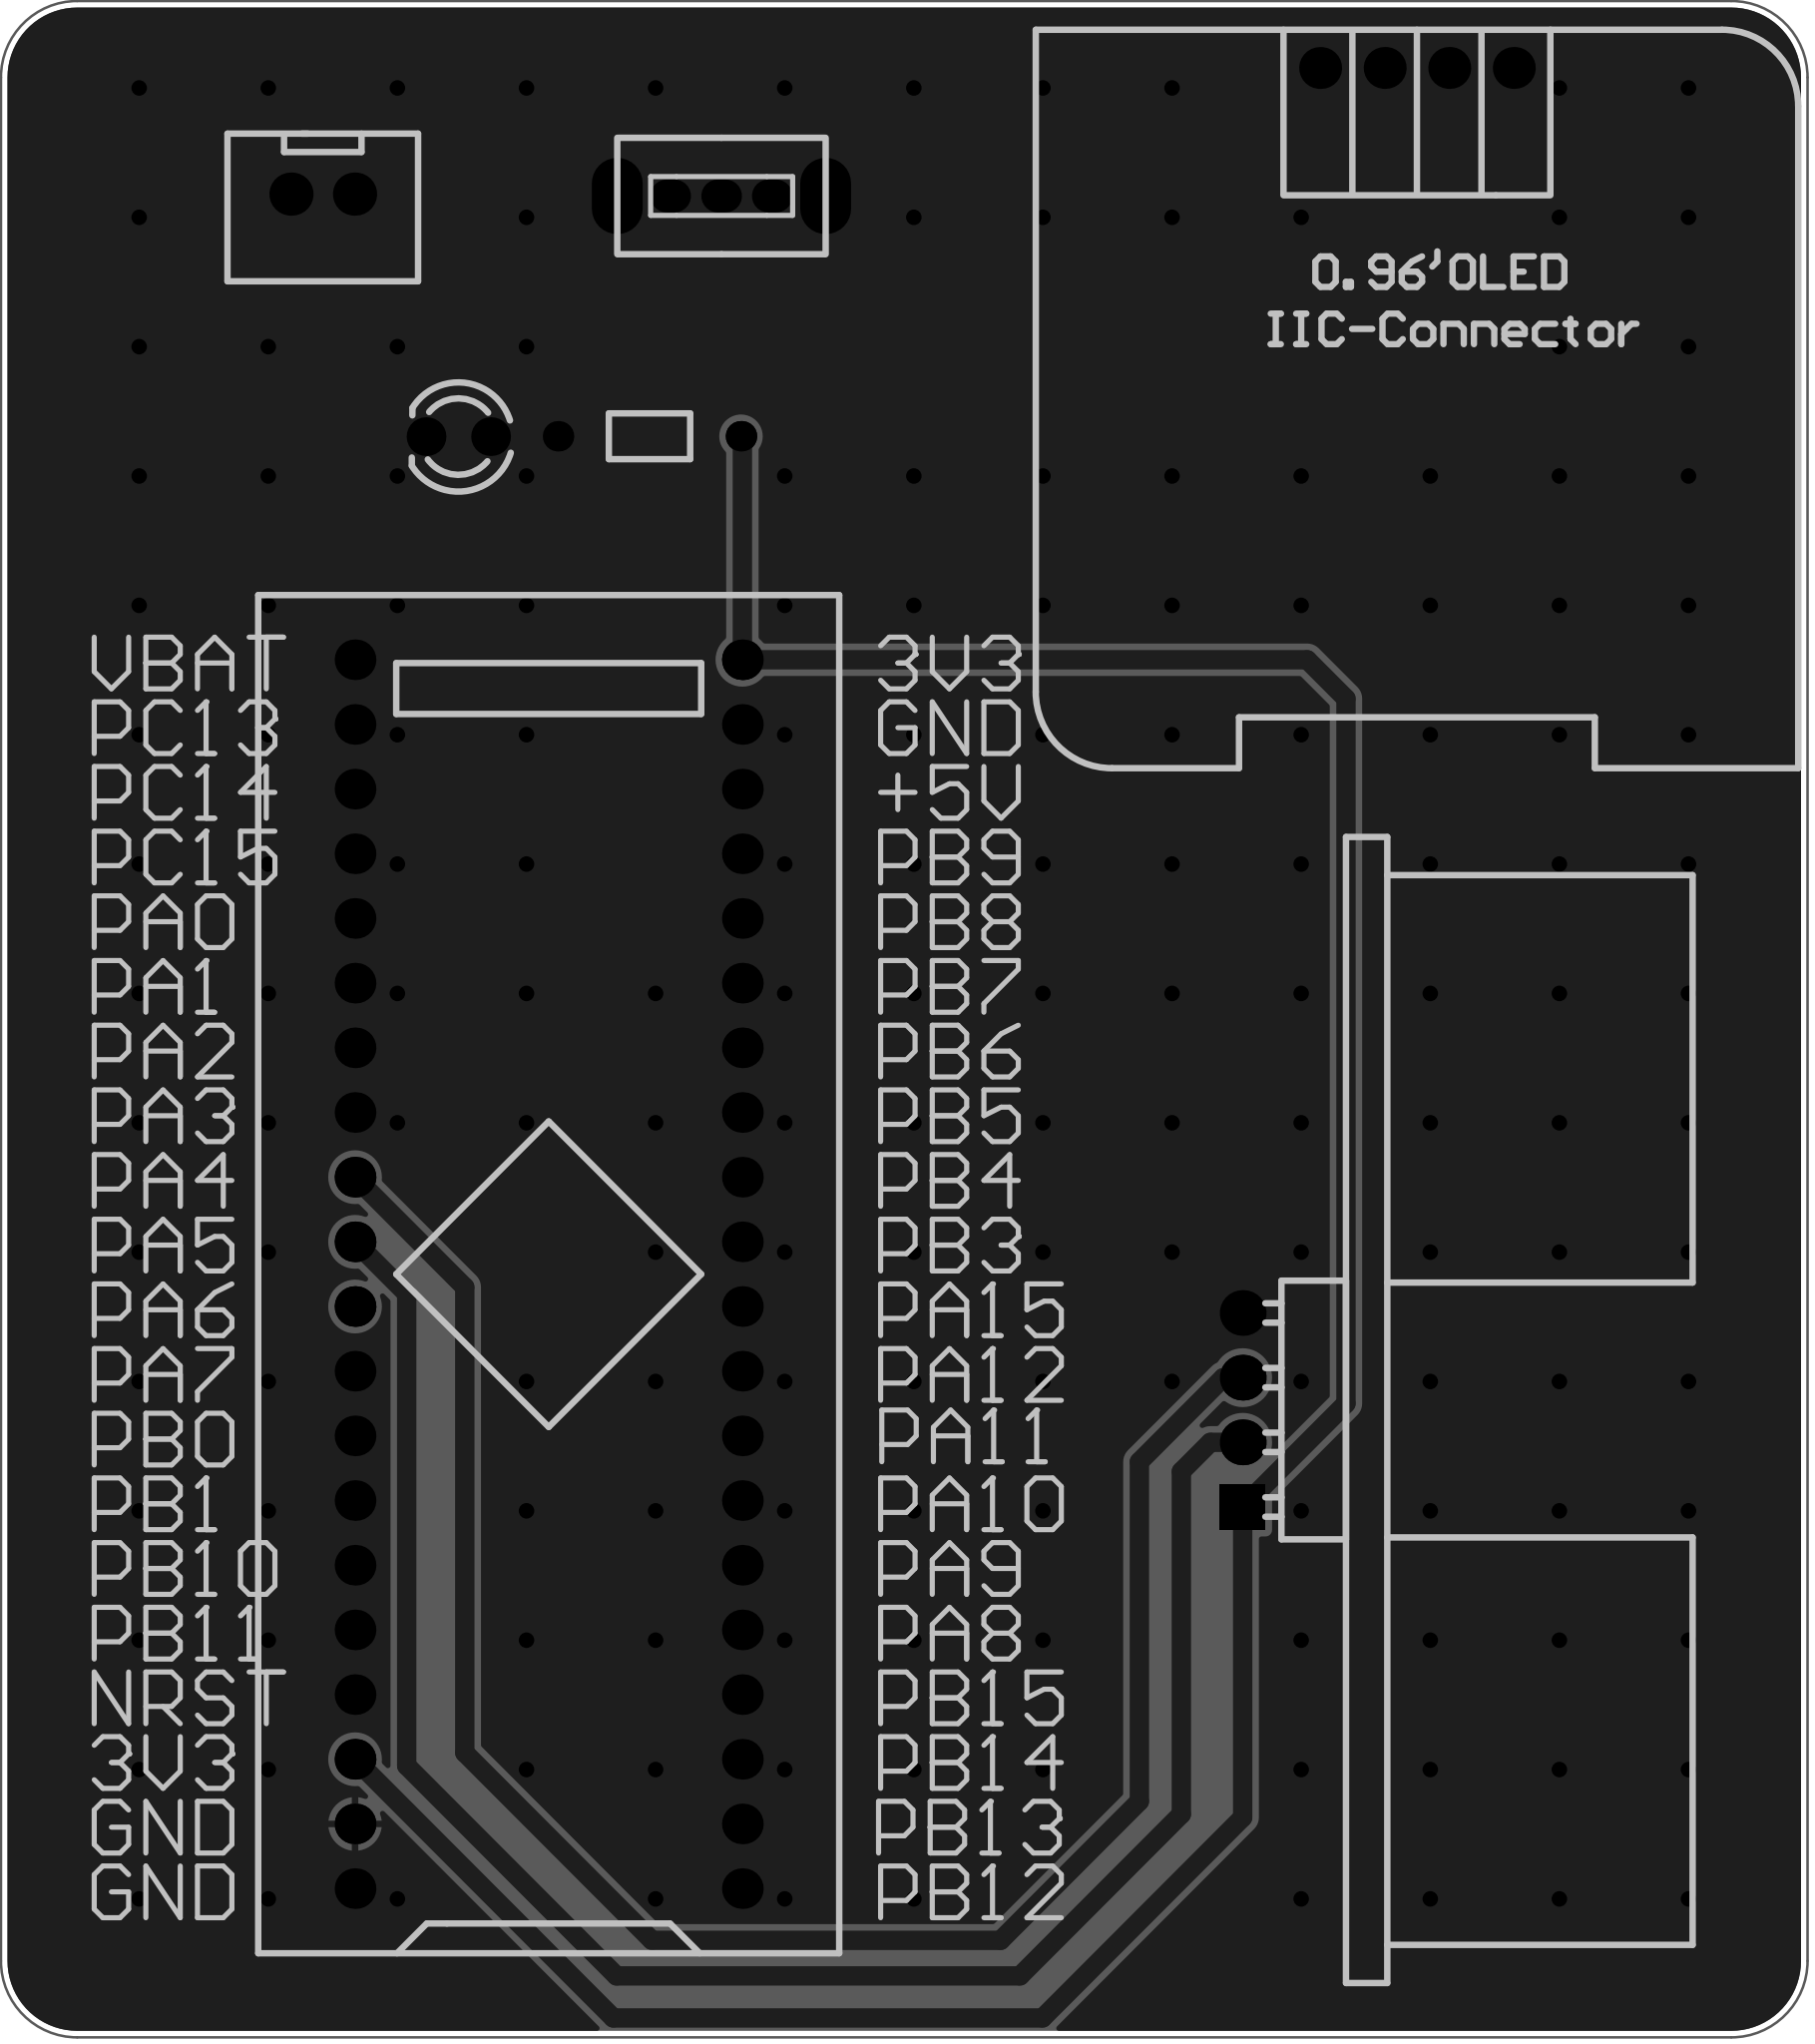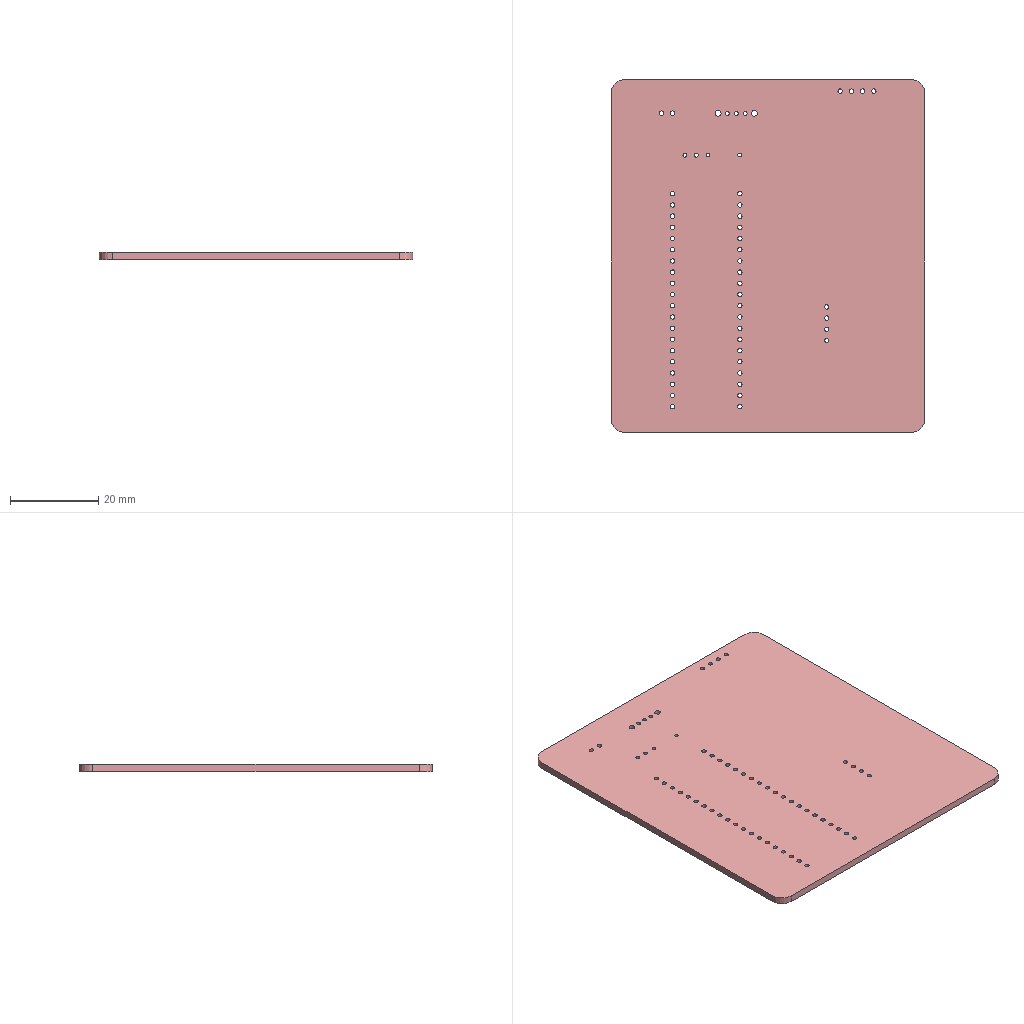Circuit board layout | Altium Designer | box 71.1 x 80 x 1.6 mm
Layer stack:
# Altium Designer layer stack of  (unit mm; dielectric type: 0 none, 1 core, 2 prepreg, 3 surface material)
index,name,kind,layer,copper_thickness_mm,dielectric_type,dielectric_thickness_mm,dielectric_material,dielectric_constant
0,Top Paste Mask Layer,other,,,,,,
1,Top Silkscreen Layer,other,,,,,,
2,Top Solder Mask Layer,dielectric,,,3,0.01,,3.3
3,Top Layer,copper,Top Layer,0.035,,,,
4,Dielectric1,dielectric,,,3,1.51,FR4,4.5
5,Bottom Layer,copper,Bottom Layer,0.035,,,,
6,Bottom Solder Mask Layer,dielectric,,,3,0.01,,3.3
7,Bottom Silkscreen Layer,other,,,,,,
8,Bottom Paste Mask Layer,other,,,,,,
# drill layer pairs: low layer,high layer
drill_pair,Top Layer,Bottom Layer
Part placement:
Designator,Comment,Layer,Footprint,Center-X(mm),Center-Y(mm),Rotation
U1,STM32F103C8T6-Card,TopLayer,CONN-TH_L53.3-W22.9_STM32F103C8T6-CARD,141.351,130.937,90
OLED1,,TopLayer,0.96OLED_4P,175.514,178.308,0
CN4,XH2.54*2P_Through-hole,TopLayer,CONN-TH_2P-P2.50-XH2.54-2P,132.461,173.355,0
SW5,,TopLayer,拨动开关,148.148,173.28,180
U2,HC-SR04,TopLayer,TH_HC-SR04V,168.656,125.603,90
LED1,,TopLayer,LED_TH-3mm,137.795,163.83,180
R1,220Ω,TopLayer,Res_1/8W,145.317,163.843,0
Pad and via stacks:
# Altium Designer via and pad stacks of  (unit mm). Each distinct definition once, with the count of objects using it.
# via: kind,start_layer,end_layer,hole_mm,diameter_mm,mode(0 simple;1 top-mid-bottom;2 full stack),diameter_per_layer,count,example_net
# pad: kind,layer,hole_mm,hole_type(0 round;1 square;2 slot),plating,top_size,top_shape(1 round;2 rect;3 octagon;9 rounded rect),mid_size,bottom_size,mode,footprint,size_per_layer,count,example
pad,Multi-Layer,1,0,plated,1.6x1.6,1,1.6x1.6,1.6x1.6,0,CONN-TH_L53.3-W22.9_STM32F103C8T6-CARD,,40,U1.1
pad,Multi-Layer,1,0,plated,1.65x1.65,1,1.65x1.65,1.65x1.65,0,0.96OLED_4P,,4,OLED1.4
pad,Multi-Layer,1.05,0,plated,1.7x1.7,1,1.7x1.7,1.7x1.7,0,CONN-TH_2P-P2.50-XH2.54-2P,,2,CN4.2
pad,Multi-Layer,0.8992,0,plated,1.6x1.3,1,1.6x1.3,1.6x1.3,0,\u00B2\u00A6\u00B6\u00AF\u00BF\u00AA\u00B9\u00D8,,3,SW5.1
pad,Multi-Layer,1.3,0,plated,3x1.999,1,3x1.999,3x1.999,0,\u00B2\u00A6\u00B6\u00AF\u00BF\u00AA\u00B9\u00D8,,2,SW5.4
pad,Multi-Layer,1.001,0,plated,1.8x1.8,1,1.8x1.8,1.8x1.8,0,TH_HC-SR04V,,3,U2.4
pad,Multi-Layer,1.001,0,plated,1.8x1.8,2,1.8x1.8,1.8x1.8,0,TH_HC-SR04V,,1,U2.1
pad,Multi-Layer,0.9144,0,plated,1.524x1.524,1,1.524x1.524,1.524x1.524,0,LED_TH-3mm,,2,LED1.1
pad,Multi-Layer,0.8001,0,plated,1.199x1.199,1,1.199x1.199,1.199x1.199,0,Res_1/8W,,2,R1.1
via,Top Layer,Bottom Layer,0.3048,0.61,0,,165,GND
Copper pours:
name,layer,net,type(0 solid;1 hatched;2 none)
Bottom Layer-GND,Bottom Layer,GND,0
Top Layer-GND,Top Layer,GND,0